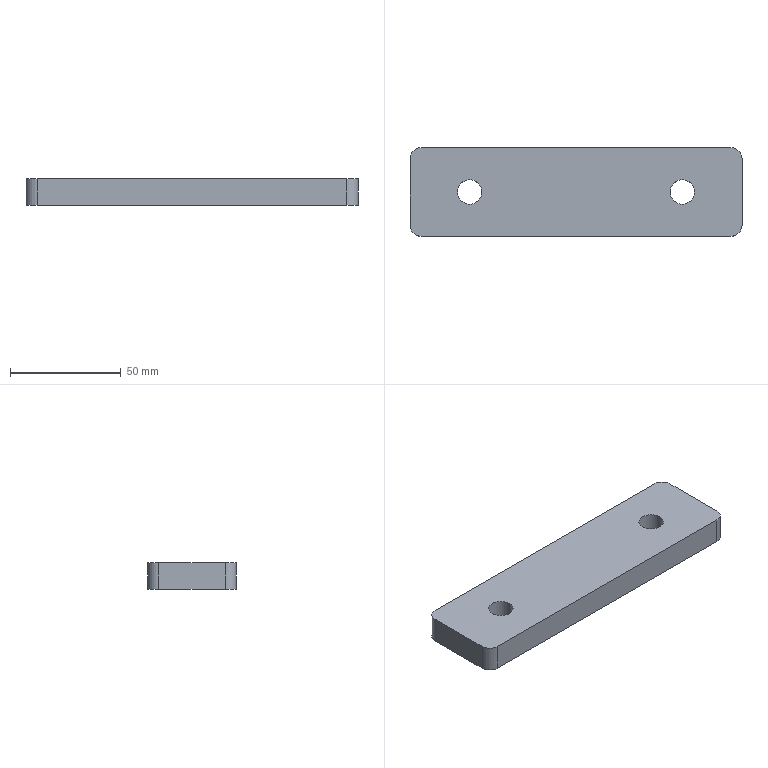Part | SolidWorks | features Cut 1, Extrusion 1, Fillet 1, ICE 1 | 1 solid | 14 faces | box 150 x 40 x 12 mm | volume 69462 mm3 | cylinder 8 | plane 6 | commonest cylinder face diameters 10 x4 11 x4
STEP:
#1=CARTESIAN_POINT('',(53.5,0.,0.));
#2=VERTEX_POINT('',#1);
#3=CARTESIAN_POINT('',(42.5,0.,0.));
#4=VERTEX_POINT('',#3);
#5=CARTESIAN_POINT('',(48.,0.,0.));
#6=DIRECTION('',(0.,0.,-1.));
#7=DIRECTION('',(-1.,0.,0.));
#8=AXIS2_PLACEMENT_3D('',#5,#6,#7);
#9=CIRCLE('',#8,5.5);
#10=EDGE_CURVE('',#2,#4,#9,.T.);
#11=ORIENTED_EDGE('',*,*,#10,.T.);
#12=CARTESIAN_POINT('',(42.5,0.,12.));
#13=VERTEX_POINT('',#12);
#14=CARTESIAN_POINT('',(42.5,0.,4.));
#15=DIRECTION('',(0.,0.,1.));
#16=VECTOR('',#15,1000.);
#17=LINE('',#14,#16);
#18=EDGE_CURVE('',#4,#13,#17,.T.);
#19=ORIENTED_EDGE('',*,*,#18,.T.);
#20=CARTESIAN_POINT('',(53.5,0.,12.));
#21=VERTEX_POINT('',#20);
#22=CARTESIAN_POINT('',(48.,0.,12.));
#23=DIRECTION('',(0.,0.,1.));
#24=DIRECTION('',(1.,0.,0.));
#25=AXIS2_PLACEMENT_3D('',#22,#23,#24);
#26=CIRCLE('',#25,5.5);
#27=EDGE_CURVE('',#13,#21,#26,.T.);
#28=ORIENTED_EDGE('',*,*,#27,.T.);
#29=CARTESIAN_POINT('',(53.5,0.,4.));
#30=DIRECTION('',(0.,0.,1.));
#31=VECTOR('',#30,1000.);
#32=LINE('',#29,#31);
#33=EDGE_CURVE('',#2,#21,#32,.T.);
#34=ORIENTED_EDGE('',*,*,#33,.F.);
#35=EDGE_LOOP('',(#11,#19,#28,#34));
#36=FACE_OUTER_BOUND('',#35,.T.);
#37=CARTESIAN_POINT('',(48.,0.,4.));
#38=DIRECTION('',(0.,0.,1.));
#39=DIRECTION('',(1.,0.,0.));
#40=AXIS2_PLACEMENT_3D('',#37,#38,#39);
#41=CYLINDRICAL_SURFACE('',#40,5.5);
#42=ADVANCED_FACE('',(#36),#41,.F.);
#43=CARTESIAN_POINT('',(-42.5,0.,0.));
#44=VERTEX_POINT('',#43);
#45=CARTESIAN_POINT('',(-53.5,0.,0.));
#46=VERTEX_POINT('',#45);
#47=CARTESIAN_POINT('',(-48.,0.,0.));
#48=DIRECTION('',(0.,0.,-1.));
#49=DIRECTION('',(-1.,0.,0.));
#50=AXIS2_PLACEMENT_3D('',#47,#48,#49);
#51=CIRCLE('',#50,5.5);
#52=EDGE_CURVE('',#44,#46,#51,.T.);
#53=ORIENTED_EDGE('',*,*,#52,.T.);
#54=CARTESIAN_POINT('',(-53.5,0.,12.));
#55=VERTEX_POINT('',#54);
#56=CARTESIAN_POINT('',(-53.5,0.,4.));
#57=DIRECTION('',(0.,0.,1.));
#58=VECTOR('',#57,1000.);
#59=LINE('',#56,#58);
#60=EDGE_CURVE('',#46,#55,#59,.T.);
#61=ORIENTED_EDGE('',*,*,#60,.T.);
#62=CARTESIAN_POINT('',(-42.5,0.,12.));
#63=VERTEX_POINT('',#62);
#64=CARTESIAN_POINT('',(-48.,0.,12.));
#65=DIRECTION('',(0.,0.,1.));
#66=DIRECTION('',(1.,0.,0.));
#67=AXIS2_PLACEMENT_3D('',#64,#65,#66);
#68=CIRCLE('',#67,5.5);
#69=EDGE_CURVE('',#55,#63,#68,.T.);
#70=ORIENTED_EDGE('',*,*,#69,.T.);
#71=CARTESIAN_POINT('',(-42.5,0.,4.));
#72=DIRECTION('',(0.,0.,1.));
#73=VECTOR('',#72,1000.);
#74=LINE('',#71,#73);
#75=EDGE_CURVE('',#44,#63,#74,.T.);
#76=ORIENTED_EDGE('',*,*,#75,.F.);
#77=EDGE_LOOP('',(#53,#61,#70,#76));
#78=FACE_OUTER_BOUND('',#77,.T.);
#79=CARTESIAN_POINT('',(-48.,0.,4.));
#80=DIRECTION('',(0.,0.,1.));
#81=DIRECTION('',(1.,0.,0.));
#82=AXIS2_PLACEMENT_3D('',#79,#80,#81);
#83=CYLINDRICAL_SURFACE('',#82,5.5);
#84=ADVANCED_FACE('',(#78),#83,.F.);
#85=CARTESIAN_POINT('',(75.,-15.,12.));
#86=VERTEX_POINT('',#85);
#87=CARTESIAN_POINT('',(75.,15.,12.));
#88=VERTEX_POINT('',#87);
#89=CARTESIAN_POINT('',(75.,-20.,12.));
#90=DIRECTION('',(0.,1.,0.));
#91=VECTOR('',#90,1000.);
#92=LINE('',#89,#91);
#93=EDGE_CURVE('',#86,#88,#92,.T.);
#94=ORIENTED_EDGE('',*,*,#93,.F.);
#95=CARTESIAN_POINT('',(75.,-15.,0.));
#96=VERTEX_POINT('',#95);
#97=CARTESIAN_POINT('',(75.,-15.,12.));
#98=DIRECTION('',(0.,0.,-1.));
#99=VECTOR('',#98,1000.);
#100=LINE('',#97,#99);
#101=EDGE_CURVE('',#86,#96,#100,.T.);
#102=ORIENTED_EDGE('',*,*,#101,.T.);
#103=CARTESIAN_POINT('',(75.,15.,0.));
#104=VERTEX_POINT('',#103);
#105=CARTESIAN_POINT('',(75.,-20.,0.));
#106=DIRECTION('',(0.,1.,0.));
#107=VECTOR('',#106,1000.);
#108=LINE('',#105,#107);
#109=EDGE_CURVE('',#96,#104,#108,.T.);
#110=ORIENTED_EDGE('',*,*,#109,.T.);
#111=CARTESIAN_POINT('',(75.,15.,12.));
#112=DIRECTION('',(0.,0.,1.));
#113=VECTOR('',#112,1000.);
#114=LINE('',#111,#113);
#115=EDGE_CURVE('',#104,#88,#114,.T.);
#116=ORIENTED_EDGE('',*,*,#115,.T.);
#117=EDGE_LOOP('',(#94,#102,#110,#116));
#118=FACE_OUTER_BOUND('',#117,.T.);
#119=CARTESIAN_POINT('',(75.,-20.,12.));
#120=DIRECTION('',(-1.,0.,0.));
#121=DIRECTION('',(0.,0.,1.));
#122=AXIS2_PLACEMENT_3D('',#119,#120,#121);
#123=PLANE('',#122);
#124=ADVANCED_FACE('',(#118),#123,.F.);
#125=CARTESIAN_POINT('',(70.,20.,12.));
#126=VERTEX_POINT('',#125);
#127=CARTESIAN_POINT('',(-70.,20.,12.));
#128=VERTEX_POINT('',#127);
#129=CARTESIAN_POINT('',(-75.,20.,12.));
#130=DIRECTION('',(-1.,0.,0.));
#131=VECTOR('',#130,1000.);
#132=LINE('',#129,#131);
#133=EDGE_CURVE('',#126,#128,#132,.T.);
#134=ORIENTED_EDGE('',*,*,#133,.F.);
#135=CARTESIAN_POINT('',(70.,20.,0.));
#136=VERTEX_POINT('',#135);
#137=CARTESIAN_POINT('',(70.,20.,12.));
#138=DIRECTION('',(0.,0.,-1.));
#139=VECTOR('',#138,1000.);
#140=LINE('',#137,#139);
#141=EDGE_CURVE('',#126,#136,#140,.T.);
#142=ORIENTED_EDGE('',*,*,#141,.T.);
#143=CARTESIAN_POINT('',(-70.,20.,0.));
#144=VERTEX_POINT('',#143);
#145=CARTESIAN_POINT('',(-75.,20.,0.));
#146=DIRECTION('',(-1.,0.,0.));
#147=VECTOR('',#146,1000.);
#148=LINE('',#145,#147);
#149=EDGE_CURVE('',#136,#144,#148,.T.);
#150=ORIENTED_EDGE('',*,*,#149,.T.);
#151=CARTESIAN_POINT('',(-70.,20.,12.));
#152=DIRECTION('',(0.,0.,1.));
#153=VECTOR('',#152,1000.);
#154=LINE('',#151,#153);
#155=EDGE_CURVE('',#144,#128,#154,.T.);
#156=ORIENTED_EDGE('',*,*,#155,.T.);
#157=EDGE_LOOP('',(#134,#142,#150,#156));
#158=FACE_OUTER_BOUND('',#157,.T.);
#159=CARTESIAN_POINT('',(-75.,20.,12.));
#160=DIRECTION('',(0.,-1.,0.));
#161=DIRECTION('',(0.,0.,-1.));
#162=AXIS2_PLACEMENT_3D('',#159,#160,#161);
#163=PLANE('',#162);
#164=ADVANCED_FACE('',(#158),#163,.F.);
#165=CARTESIAN_POINT('',(-75.,15.,0.));
#166=VERTEX_POINT('',#165);
#167=CARTESIAN_POINT('',(-75.,-15.,0.));
#168=VERTEX_POINT('',#167);
#169=CARTESIAN_POINT('',(-75.,-20.,0.));
#170=DIRECTION('',(0.,-1.,0.));
#171=VECTOR('',#170,1000.);
#172=LINE('',#169,#171);
#173=EDGE_CURVE('',#166,#168,#172,.T.);
#174=ORIENTED_EDGE('',*,*,#173,.T.);
#175=CARTESIAN_POINT('',(-75.,-15.,12.));
#176=VERTEX_POINT('',#175);
#177=CARTESIAN_POINT('',(-75.,-15.,12.));
#178=DIRECTION('',(0.,0.,1.));
#179=VECTOR('',#178,1000.);
#180=LINE('',#177,#179);
#181=EDGE_CURVE('',#168,#176,#180,.T.);
#182=ORIENTED_EDGE('',*,*,#181,.T.);
#183=CARTESIAN_POINT('',(-75.,15.,12.));
#184=VERTEX_POINT('',#183);
#185=CARTESIAN_POINT('',(-75.,-20.,12.));
#186=DIRECTION('',(0.,-1.,0.));
#187=VECTOR('',#186,1000.);
#188=LINE('',#185,#187);
#189=EDGE_CURVE('',#184,#176,#188,.T.);
#190=ORIENTED_EDGE('',*,*,#189,.F.);
#191=CARTESIAN_POINT('',(-75.,15.,12.));
#192=DIRECTION('',(0.,0.,-1.));
#193=VECTOR('',#192,1000.);
#194=LINE('',#191,#193);
#195=EDGE_CURVE('',#184,#166,#194,.T.);
#196=ORIENTED_EDGE('',*,*,#195,.T.);
#197=EDGE_LOOP('',(#174,#182,#190,#196));
#198=FACE_OUTER_BOUND('',#197,.T.);
#199=CARTESIAN_POINT('',(-75.,-20.,12.));
#200=DIRECTION('',(1.,0.,0.));
#201=DIRECTION('',(0.,0.,-1.));
#202=AXIS2_PLACEMENT_3D('',#199,#200,#201);
#203=PLANE('',#202);
#204=ADVANCED_FACE('',(#198),#203,.F.);
#205=CARTESIAN_POINT('',(-70.,-20.,0.));
#206=VERTEX_POINT('',#205);
#207=CARTESIAN_POINT('',(70.,-20.,0.));
#208=VERTEX_POINT('',#207);
#209=CARTESIAN_POINT('',(-75.,-20.,0.));
#210=DIRECTION('',(1.,0.,0.));
#211=VECTOR('',#210,1000.);
#212=LINE('',#209,#211);
#213=EDGE_CURVE('',#206,#208,#212,.T.);
#214=ORIENTED_EDGE('',*,*,#213,.T.);
#215=CARTESIAN_POINT('',(70.,-20.,12.));
#216=VERTEX_POINT('',#215);
#217=CARTESIAN_POINT('',(70.,-20.,12.));
#218=DIRECTION('',(0.,0.,1.));
#219=VECTOR('',#218,1000.);
#220=LINE('',#217,#219);
#221=EDGE_CURVE('',#208,#216,#220,.T.);
#222=ORIENTED_EDGE('',*,*,#221,.T.);
#223=CARTESIAN_POINT('',(-70.,-20.,12.));
#224=VERTEX_POINT('',#223);
#225=CARTESIAN_POINT('',(-75.,-20.,12.));
#226=DIRECTION('',(1.,0.,0.));
#227=VECTOR('',#226,1000.);
#228=LINE('',#225,#227);
#229=EDGE_CURVE('',#224,#216,#228,.T.);
#230=ORIENTED_EDGE('',*,*,#229,.F.);
#231=CARTESIAN_POINT('',(-70.,-20.,12.));
#232=DIRECTION('',(0.,0.,-1.));
#233=VECTOR('',#232,1000.);
#234=LINE('',#231,#233);
#235=EDGE_CURVE('',#224,#206,#234,.T.);
#236=ORIENTED_EDGE('',*,*,#235,.T.);
#237=EDGE_LOOP('',(#214,#222,#230,#236));
#238=FACE_OUTER_BOUND('',#237,.T.);
#239=CARTESIAN_POINT('',(-75.,-20.,12.));
#240=DIRECTION('',(0.,1.,0.));
#241=DIRECTION('',(0.,0.,1.));
#242=AXIS2_PLACEMENT_3D('',#239,#240,#241);
#243=PLANE('',#242);
#244=ADVANCED_FACE('',(#238),#243,.F.);
#245=CARTESIAN_POINT('',(48.,0.,12.));
#246=DIRECTION('',(0.,0.,1.));
#247=DIRECTION('',(1.,0.,0.));
#248=AXIS2_PLACEMENT_3D('',#245,#246,#247);
#249=CIRCLE('',#248,5.5);
#250=EDGE_CURVE('',#21,#13,#249,.T.);
#251=ORIENTED_EDGE('',*,*,#250,.F.);
#252=ORIENTED_EDGE('',*,*,#27,.F.);
#253=EDGE_LOOP('',(#251,#252));
#254=FACE_BOUND('',#253,.T.);
#255=CARTESIAN_POINT('',(-48.,0.,12.));
#256=DIRECTION('',(0.,0.,1.));
#257=DIRECTION('',(1.,0.,0.));
#258=AXIS2_PLACEMENT_3D('',#255,#256,#257);
#259=CIRCLE('',#258,5.5);
#260=EDGE_CURVE('',#63,#55,#259,.T.);
#261=ORIENTED_EDGE('',*,*,#260,.F.);
#262=ORIENTED_EDGE('',*,*,#69,.F.);
#263=EDGE_LOOP('',(#261,#262));
#264=FACE_BOUND('',#263,.T.);
#265=ORIENTED_EDGE('',*,*,#229,.T.);
#266=CARTESIAN_POINT('',(70.,-15.,12.));
#267=DIRECTION('',(0.,0.,1.));
#268=DIRECTION('',(-1.,0.,0.));
#269=AXIS2_PLACEMENT_3D('',#266,#267,#268);
#270=CIRCLE('',#269,5.);
#271=EDGE_CURVE('',#216,#86,#270,.T.);
#272=ORIENTED_EDGE('',*,*,#271,.T.);
#273=ORIENTED_EDGE('',*,*,#93,.T.);
#274=CARTESIAN_POINT('',(70.,15.,12.));
#275=DIRECTION('',(0.,0.,1.));
#276=DIRECTION('',(-1.,0.,0.));
#277=AXIS2_PLACEMENT_3D('',#274,#275,#276);
#278=CIRCLE('',#277,5.);
#279=EDGE_CURVE('',#88,#126,#278,.T.);
#280=ORIENTED_EDGE('',*,*,#279,.T.);
#281=ORIENTED_EDGE('',*,*,#133,.T.);
#282=CARTESIAN_POINT('',(-70.,15.,12.));
#283=DIRECTION('',(0.,0.,1.));
#284=DIRECTION('',(-1.,0.,0.));
#285=AXIS2_PLACEMENT_3D('',#282,#283,#284);
#286=CIRCLE('',#285,5.);
#287=EDGE_CURVE('',#128,#184,#286,.T.);
#288=ORIENTED_EDGE('',*,*,#287,.T.);
#289=ORIENTED_EDGE('',*,*,#189,.T.);
#290=CARTESIAN_POINT('',(-70.,-15.,12.));
#291=DIRECTION('',(0.,0.,1.));
#292=DIRECTION('',(-1.,0.,0.));
#293=AXIS2_PLACEMENT_3D('',#290,#291,#292);
#294=CIRCLE('',#293,5.);
#295=EDGE_CURVE('',#176,#224,#294,.T.);
#296=ORIENTED_EDGE('',*,*,#295,.T.);
#297=EDGE_LOOP('',(#265,#272,#273,#280,#281,#288,#289,#296));
#298=FACE_OUTER_BOUND('',#297,.T.);
#299=CARTESIAN_POINT('',(0.,0.,12.));
#300=DIRECTION('',(0.,0.,-1.));
#301=DIRECTION('',(-1.,0.,0.));
#302=AXIS2_PLACEMENT_3D('',#299,#300,#301);
#303=PLANE('',#302);
#304=ADVANCED_FACE('',(#254,#264,#298),#303,.F.);
#305=ORIENTED_EDGE('',*,*,#10,.F.);
#306=CARTESIAN_POINT('',(48.,0.,0.));
#307=DIRECTION('',(0.,0.,-1.));
#308=DIRECTION('',(-1.,0.,0.));
#309=AXIS2_PLACEMENT_3D('',#306,#307,#308);
#310=CIRCLE('',#309,5.5);
#311=EDGE_CURVE('',#4,#2,#310,.T.);
#312=ORIENTED_EDGE('',*,*,#311,.F.);
#313=EDGE_LOOP('',(#305,#312));
#314=FACE_BOUND('',#313,.T.);
#315=ORIENTED_EDGE('',*,*,#52,.F.);
#316=CARTESIAN_POINT('',(-48.,0.,0.));
#317=DIRECTION('',(0.,0.,-1.));
#318=DIRECTION('',(-1.,0.,0.));
#319=AXIS2_PLACEMENT_3D('',#316,#317,#318);
#320=CIRCLE('',#319,5.5);
#321=EDGE_CURVE('',#46,#44,#320,.T.);
#322=ORIENTED_EDGE('',*,*,#321,.F.);
#323=EDGE_LOOP('',(#315,#322));
#324=FACE_BOUND('',#323,.T.);
#325=ORIENTED_EDGE('',*,*,#109,.F.);
#326=CARTESIAN_POINT('',(70.,-15.,0.));
#327=DIRECTION('',(0.,0.,-1.));
#328=DIRECTION('',(-1.,0.,0.));
#329=AXIS2_PLACEMENT_3D('',#326,#327,#328);
#330=CIRCLE('',#329,5.);
#331=EDGE_CURVE('',#96,#208,#330,.T.);
#332=ORIENTED_EDGE('',*,*,#331,.T.);
#333=ORIENTED_EDGE('',*,*,#213,.F.);
#334=CARTESIAN_POINT('',(-70.,-15.,0.));
#335=DIRECTION('',(0.,0.,-1.));
#336=DIRECTION('',(-1.,0.,0.));
#337=AXIS2_PLACEMENT_3D('',#334,#335,#336);
#338=CIRCLE('',#337,5.);
#339=EDGE_CURVE('',#206,#168,#338,.T.);
#340=ORIENTED_EDGE('',*,*,#339,.T.);
#341=ORIENTED_EDGE('',*,*,#173,.F.);
#342=CARTESIAN_POINT('',(-70.,15.,0.));
#343=DIRECTION('',(0.,0.,-1.));
#344=DIRECTION('',(-1.,0.,0.));
#345=AXIS2_PLACEMENT_3D('',#342,#343,#344);
#346=CIRCLE('',#345,5.);
#347=EDGE_CURVE('',#166,#144,#346,.T.);
#348=ORIENTED_EDGE('',*,*,#347,.T.);
#349=ORIENTED_EDGE('',*,*,#149,.F.);
#350=CARTESIAN_POINT('',(70.,15.,0.));
#351=DIRECTION('',(0.,0.,-1.));
#352=DIRECTION('',(-1.,0.,0.));
#353=AXIS2_PLACEMENT_3D('',#350,#351,#352);
#354=CIRCLE('',#353,5.);
#355=EDGE_CURVE('',#136,#104,#354,.T.);
#356=ORIENTED_EDGE('',*,*,#355,.T.);
#357=EDGE_LOOP('',(#325,#332,#333,#340,#341,#348,#349,#356));
#358=FACE_OUTER_BOUND('',#357,.T.);
#359=CARTESIAN_POINT('',(0.,0.,0.));
#360=DIRECTION('',(0.,0.,-1.));
#361=DIRECTION('',(-1.,0.,0.));
#362=AXIS2_PLACEMENT_3D('',#359,#360,#361);
#363=PLANE('',#362);
#364=ADVANCED_FACE('',(#314,#324,#358),#363,.T.);
#365=ORIENTED_EDGE('',*,*,#60,.F.);
#366=ORIENTED_EDGE('',*,*,#321,.T.);
#367=ORIENTED_EDGE('',*,*,#75,.T.);
#368=ORIENTED_EDGE('',*,*,#260,.T.);
#369=EDGE_LOOP('',(#365,#366,#367,#368));
#370=FACE_OUTER_BOUND('',#369,.T.);
#371=CARTESIAN_POINT('',(-48.,0.,4.));
#372=DIRECTION('',(0.,0.,1.));
#373=DIRECTION('',(1.,0.,0.));
#374=AXIS2_PLACEMENT_3D('',#371,#372,#373);
#375=CYLINDRICAL_SURFACE('',#374,5.5);
#376=ADVANCED_FACE('',(#370),#375,.F.);
#377=ORIENTED_EDGE('',*,*,#18,.F.);
#378=ORIENTED_EDGE('',*,*,#311,.T.);
#379=ORIENTED_EDGE('',*,*,#33,.T.);
#380=ORIENTED_EDGE('',*,*,#250,.T.);
#381=EDGE_LOOP('',(#377,#378,#379,#380));
#382=FACE_OUTER_BOUND('',#381,.T.);
#383=CARTESIAN_POINT('',(48.,0.,4.));
#384=DIRECTION('',(0.,0.,1.));
#385=DIRECTION('',(1.,0.,0.));
#386=AXIS2_PLACEMENT_3D('',#383,#384,#385);
#387=CYLINDRICAL_SURFACE('',#386,5.5);
#388=ADVANCED_FACE('',(#382),#387,.F.);
#389=ORIENTED_EDGE('',*,*,#271,.F.);
#390=ORIENTED_EDGE('',*,*,#221,.F.);
#391=ORIENTED_EDGE('',*,*,#331,.F.);
#392=ORIENTED_EDGE('',*,*,#101,.F.);
#393=EDGE_LOOP('',(#389,#390,#391,#392));
#394=FACE_OUTER_BOUND('',#393,.T.);
#395=CARTESIAN_POINT('',(70.,-15.,12.));
#396=DIRECTION('',(0.,0.,-1.));
#397=DIRECTION('',(-1.,0.,0.));
#398=AXIS2_PLACEMENT_3D('',#395,#396,#397);
#399=CYLINDRICAL_SURFACE('',#398,5.);
#400=ADVANCED_FACE('',(#394),#399,.T.);
#401=ORIENTED_EDGE('',*,*,#279,.F.);
#402=ORIENTED_EDGE('',*,*,#115,.F.);
#403=ORIENTED_EDGE('',*,*,#355,.F.);
#404=ORIENTED_EDGE('',*,*,#141,.F.);
#405=EDGE_LOOP('',(#401,#402,#403,#404));
#406=FACE_OUTER_BOUND('',#405,.T.);
#407=CARTESIAN_POINT('',(70.,15.,12.));
#408=DIRECTION('',(0.,0.,-1.));
#409=DIRECTION('',(-1.,0.,0.));
#410=AXIS2_PLACEMENT_3D('',#407,#408,#409);
#411=CYLINDRICAL_SURFACE('',#410,5.);
#412=ADVANCED_FACE('',(#406),#411,.T.);
#413=ORIENTED_EDGE('',*,*,#295,.F.);
#414=ORIENTED_EDGE('',*,*,#181,.F.);
#415=ORIENTED_EDGE('',*,*,#339,.F.);
#416=ORIENTED_EDGE('',*,*,#235,.F.);
#417=EDGE_LOOP('',(#413,#414,#415,#416));
#418=FACE_OUTER_BOUND('',#417,.T.);
#419=CARTESIAN_POINT('',(-70.,-15.,12.));
#420=DIRECTION('',(0.,0.,-1.));
#421=DIRECTION('',(-1.,0.,0.));
#422=AXIS2_PLACEMENT_3D('',#419,#420,#421);
#423=CYLINDRICAL_SURFACE('',#422,5.);
#424=ADVANCED_FACE('',(#418),#423,.T.);
#425=ORIENTED_EDGE('',*,*,#287,.F.);
#426=ORIENTED_EDGE('',*,*,#155,.F.);
#427=ORIENTED_EDGE('',*,*,#347,.F.);
#428=ORIENTED_EDGE('',*,*,#195,.F.);
#429=EDGE_LOOP('',(#425,#426,#427,#428));
#430=FACE_OUTER_BOUND('',#429,.T.);
#431=CARTESIAN_POINT('',(-70.,15.,12.));
#432=DIRECTION('',(0.,0.,-1.));
#433=DIRECTION('',(-1.,0.,0.));
#434=AXIS2_PLACEMENT_3D('',#431,#432,#433);
#435=CYLINDRICAL_SURFACE('',#434,5.);
#436=ADVANCED_FACE('',(#430),#435,.T.);
#437=CLOSED_SHELL('',(#42,#84,#124,#164,#204,#244,#304,#364,#376,#388,#400,#412,#424,#436));
#438=MANIFOLD_SOLID_BREP('',#437);
#439=CARTESIAN_POINT('',(0.,0.,0.));
#440=DIRECTION('',(0.,0.,1.));
#441=DIRECTION('',(1.,0.,0.));
#442=AXIS2_PLACEMENT_3D('',#439,#440,#441);
#443=(LENGTH_UNIT()NAMED_UNIT(*)SI_UNIT(.MILLI.,.METRE.));
#444=UNCERTAINTY_MEASURE_WITH_UNIT(LENGTH_MEASURE(0.00001),#443,'','');
#445=(NAMED_UNIT(*)PLANE_ANGLE_UNIT()SI_UNIT($,.RADIAN.));
#446=(NAMED_UNIT(*)SI_UNIT($,.STERADIAN.)SOLID_ANGLE_UNIT());
#447=(GEOMETRIC_REPRESENTATION_CONTEXT(3)GLOBAL_UNCERTAINTY_ASSIGNED_CONTEXT((#444))GLOBAL_UNIT_ASSIGNED_CONTEXT((#443,#445,#446))REPRESENTATION_CONTEXT('',''));
#448=ADVANCED_BREP_SHAPE_REPRESENTATION('',(#438,#442),#447);